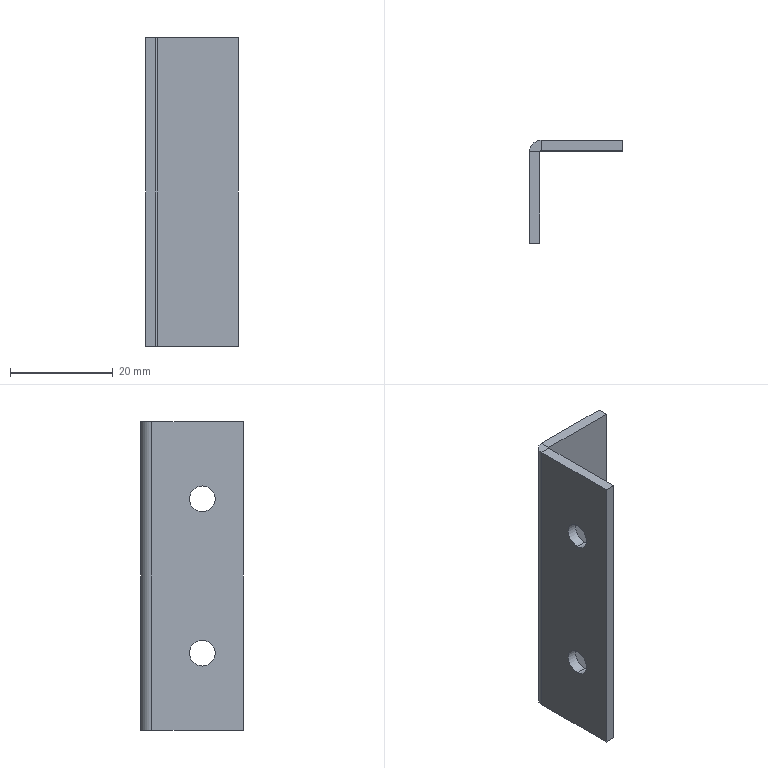Part | SolidWorks | features FlatPattern 1, ICE 1, SMBaseFlange 1, SheetMetal 1 | 1 solid | 18 faces | box 18 x 20 x 60 mm | volume 4180 mm3 | plane 12 | cylinder 6 | commonest cylinder face diameters 5 x4 0.4 x1 4.4 x1
STEP:
#1=CARTESIAN_POINT('',(-16.,-12.,17.5));
#2=VERTEX_POINT('',#1);
#3=CARTESIAN_POINT('',(-16.,-12.,12.5));
#4=VERTEX_POINT('',#3);
#5=CARTESIAN_POINT('',(-16.,-12.,15.));
#6=DIRECTION('',(1.,0.,0.));
#7=DIRECTION('',(0.,0.,-1.));
#8=AXIS2_PLACEMENT_3D('',#5,#6,#7);
#9=CIRCLE('',#8,2.5);
#10=EDGE_CURVE('',#2,#4,#9,.T.);
#11=ORIENTED_EDGE('',*,*,#10,.T.);
#12=CARTESIAN_POINT('',(-18.,-12.,12.5));
#13=VERTEX_POINT('',#12);
#14=CARTESIAN_POINT('',(-8.,-12.,12.5));
#15=DIRECTION('',(-1.,0.,0.));
#16=VECTOR('',#15,1000.);
#17=LINE('',#14,#16);
#18=EDGE_CURVE('',#4,#13,#17,.T.);
#19=ORIENTED_EDGE('',*,*,#18,.T.);
#20=CARTESIAN_POINT('',(-18.,-12.,17.5));
#21=VERTEX_POINT('',#20);
#22=CARTESIAN_POINT('',(-18.,-12.,15.));
#23=DIRECTION('',(-1.,0.,0.));
#24=DIRECTION('',(0.,0.,1.));
#25=AXIS2_PLACEMENT_3D('',#22,#23,#24);
#26=CIRCLE('',#25,2.5);
#27=EDGE_CURVE('',#13,#21,#26,.T.);
#28=ORIENTED_EDGE('',*,*,#27,.T.);
#29=CARTESIAN_POINT('',(-8.,-12.,17.5));
#30=DIRECTION('',(-1.,0.,0.));
#31=VECTOR('',#30,1000.);
#32=LINE('',#29,#31);
#33=EDGE_CURVE('',#2,#21,#32,.T.);
#34=ORIENTED_EDGE('',*,*,#33,.F.);
#35=EDGE_LOOP('',(#11,#19,#28,#34));
#36=FACE_OUTER_BOUND('',#35,.T.);
#37=CARTESIAN_POINT('',(-8.,-12.,15.));
#38=DIRECTION('',(-1.,0.,0.));
#39=DIRECTION('',(0.,0.,1.));
#40=AXIS2_PLACEMENT_3D('',#37,#38,#39);
#41=CYLINDRICAL_SURFACE('',#40,2.5);
#42=ADVANCED_FACE('',(#36),#41,.F.);
#43=CARTESIAN_POINT('',(-16.,-12.,47.5));
#44=VERTEX_POINT('',#43);
#45=CARTESIAN_POINT('',(-16.,-12.,42.5));
#46=VERTEX_POINT('',#45);
#47=CARTESIAN_POINT('',(-16.,-12.,45.));
#48=DIRECTION('',(1.,0.,0.));
#49=DIRECTION('',(0.,0.,-1.));
#50=AXIS2_PLACEMENT_3D('',#47,#48,#49);
#51=CIRCLE('',#50,2.5);
#52=EDGE_CURVE('',#44,#46,#51,.T.);
#53=ORIENTED_EDGE('',*,*,#52,.T.);
#54=CARTESIAN_POINT('',(-18.,-12.,42.5));
#55=VERTEX_POINT('',#54);
#56=CARTESIAN_POINT('',(-8.,-12.,42.5));
#57=DIRECTION('',(-1.,0.,0.));
#58=VECTOR('',#57,1000.);
#59=LINE('',#56,#58);
#60=EDGE_CURVE('',#46,#55,#59,.T.);
#61=ORIENTED_EDGE('',*,*,#60,.T.);
#62=CARTESIAN_POINT('',(-18.,-12.,47.5));
#63=VERTEX_POINT('',#62);
#64=CARTESIAN_POINT('',(-18.,-12.,45.));
#65=DIRECTION('',(-1.,0.,0.));
#66=DIRECTION('',(0.,0.,1.));
#67=AXIS2_PLACEMENT_3D('',#64,#65,#66);
#68=CIRCLE('',#67,2.5);
#69=EDGE_CURVE('',#55,#63,#68,.T.);
#70=ORIENTED_EDGE('',*,*,#69,.T.);
#71=CARTESIAN_POINT('',(-8.,-12.,47.5));
#72=DIRECTION('',(-1.,0.,0.));
#73=VECTOR('',#72,1000.);
#74=LINE('',#71,#73);
#75=EDGE_CURVE('',#44,#63,#74,.T.);
#76=ORIENTED_EDGE('',*,*,#75,.F.);
#77=EDGE_LOOP('',(#53,#61,#70,#76));
#78=FACE_OUTER_BOUND('',#77,.T.);
#79=CARTESIAN_POINT('',(-8.,-12.,45.));
#80=DIRECTION('',(-1.,0.,0.));
#81=DIRECTION('',(0.,0.,1.));
#82=AXIS2_PLACEMENT_3D('',#79,#80,#81);
#83=CYLINDRICAL_SURFACE('',#82,2.5);
#84=ADVANCED_FACE('',(#78),#83,.F.);
#85=CARTESIAN_POINT('',(-15.8,0.,60.));
#86=VERTEX_POINT('',#85);
#87=CARTESIAN_POINT('',(-15.8,-2.,60.));
#88=VERTEX_POINT('',#87);
#89=CARTESIAN_POINT('',(-15.8,0.,60.));
#90=DIRECTION('',(0.,-1.,0.));
#91=VECTOR('',#90,1000.);
#92=LINE('',#89,#91);
#93=EDGE_CURVE('',#86,#88,#92,.T.);
#94=ORIENTED_EDGE('',*,*,#93,.F.);
#95=CARTESIAN_POINT('',(-18.,-2.2,60.));
#96=VERTEX_POINT('',#95);
#97=CARTESIAN_POINT('',(-15.8,-2.2,60.));
#98=DIRECTION('',(0.,0.,1.));
#99=DIRECTION('',(-1.,0.,0.));
#100=AXIS2_PLACEMENT_3D('',#97,#98,#99);
#101=CIRCLE('',#100,2.2);
#102=EDGE_CURVE('',#86,#96,#101,.T.);
#103=ORIENTED_EDGE('',*,*,#102,.T.);
#104=CARTESIAN_POINT('',(-16.,-2.2,60.));
#105=VERTEX_POINT('',#104);
#106=CARTESIAN_POINT('',(-16.,-2.2,60.));
#107=DIRECTION('',(-1.,0.,0.));
#108=VECTOR('',#107,1000.);
#109=LINE('',#106,#108);
#110=EDGE_CURVE('',#105,#96,#109,.T.);
#111=ORIENTED_EDGE('',*,*,#110,.F.);
#112=CARTESIAN_POINT('',(-15.8,-2.2,60.));
#113=DIRECTION('',(0.,0.,1.));
#114=DIRECTION('',(1.,0.,0.));
#115=AXIS2_PLACEMENT_3D('',#112,#113,#114);
#116=CIRCLE('',#115,0.2);
#117=EDGE_CURVE('',#88,#105,#116,.T.);
#118=ORIENTED_EDGE('',*,*,#117,.F.);
#119=EDGE_LOOP('',(#94,#103,#111,#118));
#120=FACE_OUTER_BOUND('',#119,.T.);
#121=CARTESIAN_POINT('',(-15.8,0.,60.));
#122=DIRECTION('',(0.,0.,1.));
#123=DIRECTION('',(1.,0.,0.));
#124=AXIS2_PLACEMENT_3D('',#121,#122,#123);
#125=PLANE('',#124);
#126=ADVANCED_FACE('',(#120),#125,.T.);
#127=CARTESIAN_POINT('',(0.,0.,60.));
#128=VERTEX_POINT('',#127);
#129=CARTESIAN_POINT('',(0.,0.,60.));
#130=DIRECTION('',(-1.,0.,0.));
#131=VECTOR('',#130,1000.);
#132=LINE('',#129,#131);
#133=EDGE_CURVE('',#128,#86,#132,.T.);
#134=ORIENTED_EDGE('',*,*,#133,.T.);
#135=ORIENTED_EDGE('',*,*,#93,.T.);
#136=CARTESIAN_POINT('',(0.,-2.,60.));
#137=VERTEX_POINT('',#136);
#138=CARTESIAN_POINT('',(0.,-2.,60.));
#139=DIRECTION('',(-1.,0.,0.));
#140=VECTOR('',#139,1000.);
#141=LINE('',#138,#140);
#142=EDGE_CURVE('',#137,#88,#141,.T.);
#143=ORIENTED_EDGE('',*,*,#142,.F.);
#144=CARTESIAN_POINT('',(0.,0.,60.));
#145=DIRECTION('',(0.,-1.,0.));
#146=VECTOR('',#145,1000.);
#147=LINE('',#144,#146);
#148=EDGE_CURVE('',#128,#137,#147,.T.);
#149=ORIENTED_EDGE('',*,*,#148,.F.);
#150=EDGE_LOOP('',(#134,#135,#143,#149));
#151=FACE_OUTER_BOUND('',#150,.T.);
#152=CARTESIAN_POINT('',(-16.,-2.2,60.));
#153=DIRECTION('',(0.,0.,1.));
#154=DIRECTION('',(1.,0.,0.));
#155=AXIS2_PLACEMENT_3D('',#152,#153,#154);
#156=PLANE('',#155);
#157=ADVANCED_FACE('',(#151),#156,.T.);
#158=CARTESIAN_POINT('',(-18.,-2.2,0.));
#159=VERTEX_POINT('',#158);
#160=CARTESIAN_POINT('',(-16.,-2.2,0.));
#161=VERTEX_POINT('',#160);
#162=CARTESIAN_POINT('',(-18.,-2.2,0.));
#163=DIRECTION('',(1.,0.,0.));
#164=VECTOR('',#163,1000.);
#165=LINE('',#162,#164);
#166=EDGE_CURVE('',#159,#161,#165,.T.);
#167=ORIENTED_EDGE('',*,*,#166,.F.);
#168=CARTESIAN_POINT('',(-15.8,0.,0.));
#169=VERTEX_POINT('',#168);
#170=CARTESIAN_POINT('',(-15.8,-2.2,0.));
#171=DIRECTION('',(0.,0.,1.));
#172=DIRECTION('',(-1.,0.,0.));
#173=AXIS2_PLACEMENT_3D('',#170,#171,#172);
#174=CIRCLE('',#173,2.2);
#175=EDGE_CURVE('',#169,#159,#174,.T.);
#176=ORIENTED_EDGE('',*,*,#175,.F.);
#177=CARTESIAN_POINT('',(-15.8,-2.,0.));
#178=VERTEX_POINT('',#177);
#179=CARTESIAN_POINT('',(-15.8,-2.,0.));
#180=DIRECTION('',(0.,1.,0.));
#181=VECTOR('',#180,1000.);
#182=LINE('',#179,#181);
#183=EDGE_CURVE('',#178,#169,#182,.T.);
#184=ORIENTED_EDGE('',*,*,#183,.F.);
#185=CARTESIAN_POINT('',(-15.8,-2.2,0.));
#186=DIRECTION('',(0.,0.,1.));
#187=DIRECTION('',(1.,0.,0.));
#188=AXIS2_PLACEMENT_3D('',#185,#186,#187);
#189=CIRCLE('',#188,0.2);
#190=EDGE_CURVE('',#178,#161,#189,.T.);
#191=ORIENTED_EDGE('',*,*,#190,.T.);
#192=EDGE_LOOP('',(#167,#176,#184,#191));
#193=FACE_OUTER_BOUND('',#192,.T.);
#194=CARTESIAN_POINT('',(-18.,-2.2,0.));
#195=DIRECTION('',(0.,0.,-1.));
#196=DIRECTION('',(-1.,0.,0.));
#197=AXIS2_PLACEMENT_3D('',#194,#195,#196);
#198=PLANE('',#197);
#199=ADVANCED_FACE('',(#193),#198,.T.);
#200=CARTESIAN_POINT('',(-18.,-20.,0.));
#201=VERTEX_POINT('',#200);
#202=CARTESIAN_POINT('',(-18.,0.,0.));
#203=DIRECTION('',(0.,-1.,0.));
#204=VECTOR('',#203,1000.);
#205=LINE('',#202,#204);
#206=EDGE_CURVE('',#159,#201,#205,.T.);
#207=ORIENTED_EDGE('',*,*,#206,.F.);
#208=ORIENTED_EDGE('',*,*,#166,.T.);
#209=CARTESIAN_POINT('',(-16.,-20.,0.));
#210=VERTEX_POINT('',#209);
#211=CARTESIAN_POINT('',(-16.,0.,0.));
#212=DIRECTION('',(0.,-1.,0.));
#213=VECTOR('',#212,1000.);
#214=LINE('',#211,#213);
#215=EDGE_CURVE('',#161,#210,#214,.T.);
#216=ORIENTED_EDGE('',*,*,#215,.T.);
#217=CARTESIAN_POINT('',(-16.,-20.,0.));
#218=DIRECTION('',(-1.,0.,0.));
#219=VECTOR('',#218,1000.);
#220=LINE('',#217,#219);
#221=EDGE_CURVE('',#210,#201,#220,.T.);
#222=ORIENTED_EDGE('',*,*,#221,.T.);
#223=EDGE_LOOP('',(#207,#208,#216,#222));
#224=FACE_OUTER_BOUND('',#223,.T.);
#225=CARTESIAN_POINT('',(-15.8,-2.,0.));
#226=DIRECTION('',(0.,0.,-1.));
#227=DIRECTION('',(-1.,0.,0.));
#228=AXIS2_PLACEMENT_3D('',#225,#226,#227);
#229=PLANE('',#228);
#230=ADVANCED_FACE('',(#224),#229,.T.);
#231=CARTESIAN_POINT('',(-18.,-12.,15.));
#232=DIRECTION('',(-1.,0.,0.));
#233=DIRECTION('',(0.,0.,1.));
#234=AXIS2_PLACEMENT_3D('',#231,#232,#233);
#235=CIRCLE('',#234,2.5);
#236=EDGE_CURVE('',#21,#13,#235,.T.);
#237=ORIENTED_EDGE('',*,*,#236,.F.);
#238=ORIENTED_EDGE('',*,*,#27,.F.);
#239=EDGE_LOOP('',(#237,#238));
#240=FACE_BOUND('',#239,.T.);
#241=CARTESIAN_POINT('',(-18.,-12.,45.));
#242=DIRECTION('',(-1.,0.,0.));
#243=DIRECTION('',(0.,0.,1.));
#244=AXIS2_PLACEMENT_3D('',#241,#242,#243);
#245=CIRCLE('',#244,2.5);
#246=EDGE_CURVE('',#63,#55,#245,.T.);
#247=ORIENTED_EDGE('',*,*,#246,.F.);
#248=ORIENTED_EDGE('',*,*,#69,.F.);
#249=EDGE_LOOP('',(#247,#248));
#250=FACE_BOUND('',#249,.T.);
#251=ORIENTED_EDGE('',*,*,#206,.T.);
#252=CARTESIAN_POINT('',(-18.,-20.,60.));
#253=VERTEX_POINT('',#252);
#254=CARTESIAN_POINT('',(-18.,-20.,60.));
#255=DIRECTION('',(0.,0.,-1.));
#256=VECTOR('',#255,1000.);
#257=LINE('',#254,#256);
#258=EDGE_CURVE('',#253,#201,#257,.T.);
#259=ORIENTED_EDGE('',*,*,#258,.F.);
#260=CARTESIAN_POINT('',(-18.,0.,60.));
#261=DIRECTION('',(0.,-1.,0.));
#262=VECTOR('',#261,1000.);
#263=LINE('',#260,#262);
#264=EDGE_CURVE('',#96,#253,#263,.T.);
#265=ORIENTED_EDGE('',*,*,#264,.F.);
#266=CARTESIAN_POINT('',(-18.,-2.2,60.));
#267=DIRECTION('',(0.,0.,-1.));
#268=VECTOR('',#267,1000.);
#269=LINE('',#266,#268);
#270=EDGE_CURVE('',#96,#159,#269,.T.);
#271=ORIENTED_EDGE('',*,*,#270,.T.);
#272=EDGE_LOOP('',(#251,#259,#265,#271));
#273=FACE_OUTER_BOUND('',#272,.T.);
#274=CARTESIAN_POINT('',(-18.,0.,60.));
#275=DIRECTION('',(1.,0.,0.));
#276=DIRECTION('',(0.,0.,-1.));
#277=AXIS2_PLACEMENT_3D('',#274,#275,#276);
#278=PLANE('',#277);
#279=ADVANCED_FACE('',(#240,#250,#273),#278,.F.);
#280=ORIENTED_EDGE('',*,*,#221,.F.);
#281=CARTESIAN_POINT('',(-16.,-20.,60.));
#282=VERTEX_POINT('',#281);
#283=CARTESIAN_POINT('',(-16.,-20.,60.));
#284=DIRECTION('',(0.,0.,-1.));
#285=VECTOR('',#284,1000.);
#286=LINE('',#283,#285);
#287=EDGE_CURVE('',#282,#210,#286,.T.);
#288=ORIENTED_EDGE('',*,*,#287,.F.);
#289=CARTESIAN_POINT('',(-16.,-20.,60.));
#290=DIRECTION('',(-1.,0.,0.));
#291=VECTOR('',#290,1000.);
#292=LINE('',#289,#291);
#293=EDGE_CURVE('',#282,#253,#292,.T.);
#294=ORIENTED_EDGE('',*,*,#293,.T.);
#295=ORIENTED_EDGE('',*,*,#258,.T.);
#296=EDGE_LOOP('',(#280,#288,#294,#295));
#297=FACE_OUTER_BOUND('',#296,.T.);
#298=CARTESIAN_POINT('',(-16.,-20.,60.));
#299=DIRECTION('',(0.,-1.,0.));
#300=DIRECTION('',(0.,0.,-1.));
#301=AXIS2_PLACEMENT_3D('',#298,#299,#300);
#302=PLANE('',#301);
#303=ADVANCED_FACE('',(#297),#302,.T.);
#304=ORIENTED_EDGE('',*,*,#10,.F.);
#305=CARTESIAN_POINT('',(-16.,-12.,15.));
#306=DIRECTION('',(1.,0.,0.));
#307=DIRECTION('',(0.,0.,-1.));
#308=AXIS2_PLACEMENT_3D('',#305,#306,#307);
#309=CIRCLE('',#308,2.5);
#310=EDGE_CURVE('',#4,#2,#309,.T.);
#311=ORIENTED_EDGE('',*,*,#310,.F.);
#312=EDGE_LOOP('',(#304,#311));
#313=FACE_BOUND('',#312,.T.);
#314=ORIENTED_EDGE('',*,*,#52,.F.);
#315=CARTESIAN_POINT('',(-16.,-12.,45.));
#316=DIRECTION('',(1.,0.,0.));
#317=DIRECTION('',(0.,0.,-1.));
#318=AXIS2_PLACEMENT_3D('',#315,#316,#317);
#319=CIRCLE('',#318,2.5);
#320=EDGE_CURVE('',#46,#44,#319,.T.);
#321=ORIENTED_EDGE('',*,*,#320,.F.);
#322=EDGE_LOOP('',(#314,#321));
#323=FACE_BOUND('',#322,.T.);
#324=ORIENTED_EDGE('',*,*,#215,.F.);
#325=CARTESIAN_POINT('',(-16.,-2.2,60.));
#326=DIRECTION('',(0.,0.,-1.));
#327=VECTOR('',#326,1000.);
#328=LINE('',#325,#327);
#329=EDGE_CURVE('',#105,#161,#328,.T.);
#330=ORIENTED_EDGE('',*,*,#329,.F.);
#331=CARTESIAN_POINT('',(-16.,0.,60.));
#332=DIRECTION('',(0.,-1.,0.));
#333=VECTOR('',#332,1000.);
#334=LINE('',#331,#333);
#335=EDGE_CURVE('',#105,#282,#334,.T.);
#336=ORIENTED_EDGE('',*,*,#335,.T.);
#337=ORIENTED_EDGE('',*,*,#287,.T.);
#338=EDGE_LOOP('',(#324,#330,#336,#337));
#339=FACE_OUTER_BOUND('',#338,.T.);
#340=CARTESIAN_POINT('',(-16.,0.,60.));
#341=DIRECTION('',(1.,0.,0.));
#342=DIRECTION('',(0.,0.,-1.));
#343=AXIS2_PLACEMENT_3D('',#340,#341,#342);
#344=PLANE('',#343);
#345=ADVANCED_FACE('',(#313,#323,#339),#344,.T.);
#346=ORIENTED_EDGE('',*,*,#190,.F.);
#347=CARTESIAN_POINT('',(-15.8,-2.,60.));
#348=DIRECTION('',(0.,0.,-1.));
#349=VECTOR('',#348,1000.);
#350=LINE('',#347,#349);
#351=EDGE_CURVE('',#88,#178,#350,.T.);
#352=ORIENTED_EDGE('',*,*,#351,.F.);
#353=ORIENTED_EDGE('',*,*,#117,.T.);
#354=ORIENTED_EDGE('',*,*,#329,.T.);
#355=EDGE_LOOP('',(#346,#352,#353,#354));
#356=FACE_OUTER_BOUND('',#355,.T.);
#357=CARTESIAN_POINT('',(-15.8,-2.2,60.));
#358=DIRECTION('',(0.,0.,-1.));
#359=DIRECTION('',(-1.,0.,0.));
#360=AXIS2_PLACEMENT_3D('',#357,#358,#359);
#361=CYLINDRICAL_SURFACE('',#360,0.2);
#362=ADVANCED_FACE('',(#356),#361,.F.);
#363=CARTESIAN_POINT('',(0.,-2.,0.));
#364=VERTEX_POINT('',#363);
#365=CARTESIAN_POINT('',(0.,-2.,0.));
#366=DIRECTION('',(-1.,0.,0.));
#367=VECTOR('',#366,1000.);
#368=LINE('',#365,#367);
#369=EDGE_CURVE('',#364,#178,#368,.T.);
#370=ORIENTED_EDGE('',*,*,#369,.F.);
#371=CARTESIAN_POINT('',(0.,-2.,60.));
#372=DIRECTION('',(0.,0.,-1.));
#373=VECTOR('',#372,1000.);
#374=LINE('',#371,#373);
#375=EDGE_CURVE('',#137,#364,#374,.T.);
#376=ORIENTED_EDGE('',*,*,#375,.F.);
#377=ORIENTED_EDGE('',*,*,#142,.T.);
#378=ORIENTED_EDGE('',*,*,#351,.T.);
#379=EDGE_LOOP('',(#370,#376,#377,#378));
#380=FACE_OUTER_BOUND('',#379,.T.);
#381=CARTESIAN_POINT('',(0.,-2.,60.));
#382=DIRECTION('',(0.,-1.,0.));
#383=DIRECTION('',(1.,0.,0.));
#384=AXIS2_PLACEMENT_3D('',#381,#382,#383);
#385=PLANE('',#384);
#386=ADVANCED_FACE('',(#380),#385,.T.);
#387=CARTESIAN_POINT('',(0.,0.,0.));
#388=VERTEX_POINT('',#387);
#389=CARTESIAN_POINT('',(0.,0.,0.));
#390=DIRECTION('',(0.,-1.,0.));
#391=VECTOR('',#390,1000.);
#392=LINE('',#389,#391);
#393=EDGE_CURVE('',#388,#364,#392,.T.);
#394=ORIENTED_EDGE('',*,*,#393,.F.);
#395=CARTESIAN_POINT('',(0.,0.,60.));
#396=DIRECTION('',(0.,0.,-1.));
#397=VECTOR('',#396,1000.);
#398=LINE('',#395,#397);
#399=EDGE_CURVE('',#128,#388,#398,.T.);
#400=ORIENTED_EDGE('',*,*,#399,.F.);
#401=ORIENTED_EDGE('',*,*,#148,.T.);
#402=ORIENTED_EDGE('',*,*,#375,.T.);
#403=EDGE_LOOP('',(#394,#400,#401,#402));
#404=FACE_OUTER_BOUND('',#403,.T.);
#405=CARTESIAN_POINT('',(0.,0.,60.));
#406=DIRECTION('',(1.,0.,0.));
#407=DIRECTION('',(0.,1.,0.));
#408=AXIS2_PLACEMENT_3D('',#405,#406,#407);
#409=PLANE('',#408);
#410=ADVANCED_FACE('',(#404),#409,.T.);
#411=CARTESIAN_POINT('',(0.,0.,0.));
#412=DIRECTION('',(-1.,0.,0.));
#413=VECTOR('',#412,1000.);
#414=LINE('',#411,#413);
#415=EDGE_CURVE('',#388,#169,#414,.T.);
#416=ORIENTED_EDGE('',*,*,#415,.T.);
#417=CARTESIAN_POINT('',(-15.8,0.,60.));
#418=DIRECTION('',(0.,0.,-1.));
#419=VECTOR('',#418,1000.);
#420=LINE('',#417,#419);
#421=EDGE_CURVE('',#86,#169,#420,.T.);
#422=ORIENTED_EDGE('',*,*,#421,.F.);
#423=ORIENTED_EDGE('',*,*,#133,.F.);
#424=ORIENTED_EDGE('',*,*,#399,.T.);
#425=EDGE_LOOP('',(#416,#422,#423,#424));
#426=FACE_OUTER_BOUND('',#425,.T.);
#427=CARTESIAN_POINT('',(0.,0.,60.));
#428=DIRECTION('',(0.,-1.,0.));
#429=DIRECTION('',(1.,0.,0.));
#430=AXIS2_PLACEMENT_3D('',#427,#428,#429);
#431=PLANE('',#430);
#432=ADVANCED_FACE('',(#426),#431,.F.);
#433=ORIENTED_EDGE('',*,*,#175,.T.);
#434=ORIENTED_EDGE('',*,*,#270,.F.);
#435=ORIENTED_EDGE('',*,*,#102,.F.);
#436=ORIENTED_EDGE('',*,*,#421,.T.);
#437=EDGE_LOOP('',(#433,#434,#435,#436));
#438=FACE_OUTER_BOUND('',#437,.T.);
#439=CARTESIAN_POINT('',(-15.8,-2.2,60.));
#440=DIRECTION('',(0.,0.,-1.));
#441=DIRECTION('',(-1.,0.,0.));
#442=AXIS2_PLACEMENT_3D('',#439,#440,#441);
#443=CYLINDRICAL_SURFACE('',#442,2.2);
#444=ADVANCED_FACE('',(#438),#443,.T.);
#445=ORIENTED_EDGE('',*,*,#264,.T.);
#446=ORIENTED_EDGE('',*,*,#293,.F.);
#447=ORIENTED_EDGE('',*,*,#335,.F.);
#448=ORIENTED_EDGE('',*,*,#110,.T.);
#449=EDGE_LOOP('',(#445,#446,#447,#448));
#450=FACE_OUTER_BOUND('',#449,.T.);
#451=CARTESIAN_POINT('',(-15.8,-2.2,60.));
#452=DIRECTION('',(0.,0.,1.));
#453=DIRECTION('',(1.,0.,0.));
#454=AXIS2_PLACEMENT_3D('',#451,#452,#453);
#455=PLANE('',#454);
#456=ADVANCED_FACE('',(#450),#455,.T.);
#457=ORIENTED_EDGE('',*,*,#369,.T.);
#458=ORIENTED_EDGE('',*,*,#183,.T.);
#459=ORIENTED_EDGE('',*,*,#415,.F.);
#460=ORIENTED_EDGE('',*,*,#393,.T.);
#461=EDGE_LOOP('',(#457,#458,#459,#460));
#462=FACE_OUTER_BOUND('',#461,.T.);
#463=CARTESIAN_POINT('',(-15.8,-2.2,0.));
#464=DIRECTION('',(0.,0.,1.));
#465=DIRECTION('',(1.,0.,0.));
#466=AXIS2_PLACEMENT_3D('',#463,#464,#465);
#467=PLANE('',#466);
#468=ADVANCED_FACE('',(#462),#467,.F.);
#469=ORIENTED_EDGE('',*,*,#60,.F.);
#470=ORIENTED_EDGE('',*,*,#320,.T.);
#471=ORIENTED_EDGE('',*,*,#75,.T.);
#472=ORIENTED_EDGE('',*,*,#246,.T.);
#473=EDGE_LOOP('',(#469,#470,#471,#472));
#474=FACE_OUTER_BOUND('',#473,.T.);
#475=CARTESIAN_POINT('',(-8.,-12.,45.));
#476=DIRECTION('',(-1.,0.,0.));
#477=DIRECTION('',(0.,0.,1.));
#478=AXIS2_PLACEMENT_3D('',#475,#476,#477);
#479=CYLINDRICAL_SURFACE('',#478,2.5);
#480=ADVANCED_FACE('',(#474),#479,.F.);
#481=ORIENTED_EDGE('',*,*,#18,.F.);
#482=ORIENTED_EDGE('',*,*,#310,.T.);
#483=ORIENTED_EDGE('',*,*,#33,.T.);
#484=ORIENTED_EDGE('',*,*,#236,.T.);
#485=EDGE_LOOP('',(#481,#482,#483,#484));
#486=FACE_OUTER_BOUND('',#485,.T.);
#487=CARTESIAN_POINT('',(-8.,-12.,15.));
#488=DIRECTION('',(-1.,0.,0.));
#489=DIRECTION('',(0.,0.,1.));
#490=AXIS2_PLACEMENT_3D('',#487,#488,#489);
#491=CYLINDRICAL_SURFACE('',#490,2.5);
#492=ADVANCED_FACE('',(#486),#491,.F.);
#493=CLOSED_SHELL('',(#42,#84,#126,#157,#199,#230,#279,#303,#345,#362,#386,#410,#432,#444,#456,#468,#480,#492));
#494=MANIFOLD_SOLID_BREP('',#493);
#495=CARTESIAN_POINT('',(0.,0.,0.));
#496=DIRECTION('',(0.,0.,1.));
#497=DIRECTION('',(1.,0.,0.));
#498=AXIS2_PLACEMENT_3D('',#495,#496,#497);
#499=(LENGTH_UNIT()NAMED_UNIT(*)SI_UNIT(.MILLI.,.METRE.));
#500=UNCERTAINTY_MEASURE_WITH_UNIT(LENGTH_MEASURE(0.00001),#499,'','');
#501=(NAMED_UNIT(*)PLANE_ANGLE_UNIT()SI_UNIT($,.RADIAN.));
#502=(NAMED_UNIT(*)SI_UNIT($,.STERADIAN.)SOLID_ANGLE_UNIT());
#503=(GEOMETRIC_REPRESENTATION_CONTEXT(3)GLOBAL_UNCERTAINTY_ASSIGNED_CONTEXT((#500))GLOBAL_UNIT_ASSIGNED_CONTEXT((#499,#501,#502))REPRESENTATION_CONTEXT('',''));
#504=ADVANCED_BREP_SHAPE_REPRESENTATION('',(#494,#498),#503);